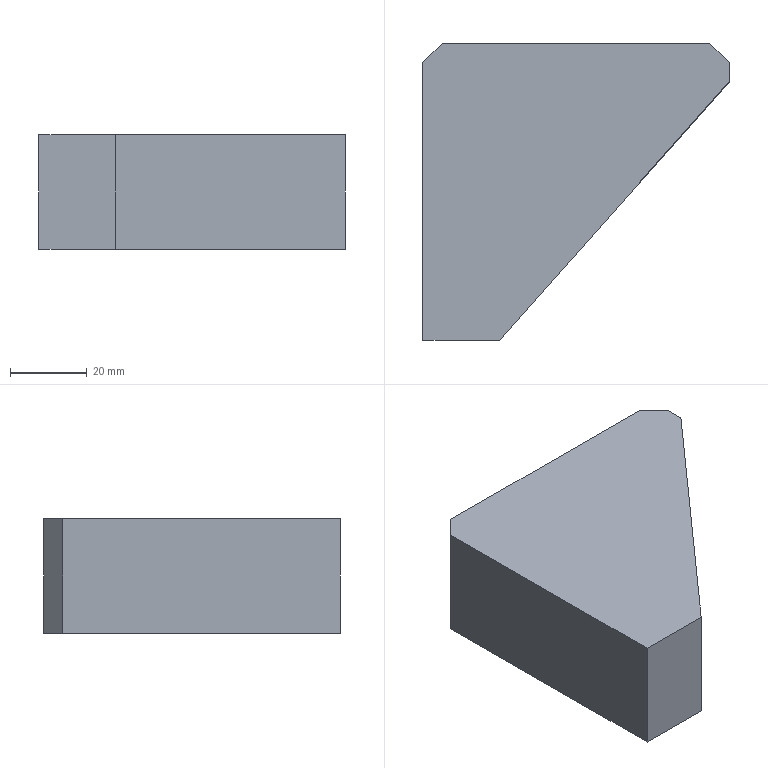Part | SolidWorks | features Extrusion 1 | 1 solid | 9 faces | box 80 x 77.5 x 30 mm | volume 124500 mm3 | plane 9
STEP:
#1=CARTESIAN_POINT('',(0.,0.,0.));
#2=VERTEX_POINT('',#1);
#3=CARTESIAN_POINT('',(20.,0.,0.));
#4=VERTEX_POINT('',#3);
#5=CARTESIAN_POINT('',(20.,0.,0.));
#6=DIRECTION('',(1.,0.,0.));
#7=VECTOR('',#6,1000.);
#8=LINE('',#5,#7);
#9=EDGE_CURVE('',#2,#4,#8,.T.);
#10=ORIENTED_EDGE('',*,*,#9,.T.);
#11=CARTESIAN_POINT('',(20.,0.,30.));
#12=VERTEX_POINT('',#11);
#13=CARTESIAN_POINT('',(20.,0.,30.));
#14=DIRECTION('',(0.,0.,-1.));
#15=VECTOR('',#14,1000.);
#16=LINE('',#13,#15);
#17=EDGE_CURVE('',#12,#4,#16,.T.);
#18=ORIENTED_EDGE('',*,*,#17,.F.);
#19=CARTESIAN_POINT('',(0.,0.,30.));
#20=VERTEX_POINT('',#19);
#21=CARTESIAN_POINT('',(20.,0.,30.));
#22=DIRECTION('',(1.,0.,0.));
#23=VECTOR('',#22,1000.);
#24=LINE('',#21,#23);
#25=EDGE_CURVE('',#20,#12,#24,.T.);
#26=ORIENTED_EDGE('',*,*,#25,.F.);
#27=CARTESIAN_POINT('',(0.,0.,30.));
#28=DIRECTION('',(0.,0.,-1.));
#29=VECTOR('',#28,1000.);
#30=LINE('',#27,#29);
#31=EDGE_CURVE('',#20,#2,#30,.T.);
#32=ORIENTED_EDGE('',*,*,#31,.T.);
#33=EDGE_LOOP('',(#10,#18,#26,#32));
#34=FACE_OUTER_BOUND('',#33,.T.);
#35=CARTESIAN_POINT('',(20.,0.,30.));
#36=DIRECTION('',(0.,1.,0.));
#37=DIRECTION('',(-1.,0.,0.));
#38=AXIS2_PLACEMENT_3D('',#35,#36,#37);
#39=PLANE('',#38);
#40=ADVANCED_FACE('',(#34),#39,.F.);
#41=CARTESIAN_POINT('',(80.,67.5,0.));
#42=VERTEX_POINT('',#41);
#43=CARTESIAN_POINT('',(80.,67.5,0.));
#44=DIRECTION('',(0.6644,0.7474,0.));
#45=VECTOR('',#44,1000.);
#46=LINE('',#43,#45);
#47=EDGE_CURVE('',#4,#42,#46,.T.);
#48=ORIENTED_EDGE('',*,*,#47,.T.);
#49=CARTESIAN_POINT('',(80.,67.5,30.));
#50=VERTEX_POINT('',#49);
#51=CARTESIAN_POINT('',(80.,67.5,30.));
#52=DIRECTION('',(0.,0.,-1.));
#53=VECTOR('',#52,1000.);
#54=LINE('',#51,#53);
#55=EDGE_CURVE('',#50,#42,#54,.T.);
#56=ORIENTED_EDGE('',*,*,#55,.F.);
#57=CARTESIAN_POINT('',(80.,67.5,30.));
#58=DIRECTION('',(0.6644,0.7474,0.));
#59=VECTOR('',#58,1000.);
#60=LINE('',#57,#59);
#61=EDGE_CURVE('',#12,#50,#60,.T.);
#62=ORIENTED_EDGE('',*,*,#61,.F.);
#63=ORIENTED_EDGE('',*,*,#17,.T.);
#64=EDGE_LOOP('',(#48,#56,#62,#63));
#65=FACE_OUTER_BOUND('',#64,.T.);
#66=CARTESIAN_POINT('',(80.,67.5,30.));
#67=DIRECTION('',(-0.7474,0.6644,0.));
#68=DIRECTION('',(-0.6644,-0.7474,0.));
#69=AXIS2_PLACEMENT_3D('',#66,#67,#68);
#70=PLANE('',#69);
#71=ADVANCED_FACE('',(#65),#70,.F.);
#72=CARTESIAN_POINT('',(80.,72.5,0.));
#73=VERTEX_POINT('',#72);
#74=CARTESIAN_POINT('',(80.,72.5,0.));
#75=DIRECTION('',(0.,1.,0.));
#76=VECTOR('',#75,1000.);
#77=LINE('',#74,#76);
#78=EDGE_CURVE('',#42,#73,#77,.T.);
#79=ORIENTED_EDGE('',*,*,#78,.T.);
#80=CARTESIAN_POINT('',(80.,72.5,30.));
#81=VERTEX_POINT('',#80);
#82=CARTESIAN_POINT('',(80.,72.5,30.));
#83=DIRECTION('',(0.,0.,-1.));
#84=VECTOR('',#83,1000.);
#85=LINE('',#82,#84);
#86=EDGE_CURVE('',#81,#73,#85,.T.);
#87=ORIENTED_EDGE('',*,*,#86,.F.);
#88=CARTESIAN_POINT('',(80.,72.5,30.));
#89=DIRECTION('',(0.,1.,0.));
#90=VECTOR('',#89,1000.);
#91=LINE('',#88,#90);
#92=EDGE_CURVE('',#50,#81,#91,.T.);
#93=ORIENTED_EDGE('',*,*,#92,.F.);
#94=ORIENTED_EDGE('',*,*,#55,.T.);
#95=EDGE_LOOP('',(#79,#87,#93,#94));
#96=FACE_OUTER_BOUND('',#95,.T.);
#97=CARTESIAN_POINT('',(80.,72.5,30.));
#98=DIRECTION('',(-1.,0.,0.));
#99=DIRECTION('',(0.,0.,1.));
#100=AXIS2_PLACEMENT_3D('',#97,#98,#99);
#101=PLANE('',#100);
#102=ADVANCED_FACE('',(#96),#101,.F.);
#103=CARTESIAN_POINT('',(75.,77.5,0.));
#104=VERTEX_POINT('',#103);
#105=CARTESIAN_POINT('',(75.,77.5,0.));
#106=DIRECTION('',(-0.7071,0.7071,0.));
#107=VECTOR('',#106,1000.);
#108=LINE('',#105,#107);
#109=EDGE_CURVE('',#73,#104,#108,.T.);
#110=ORIENTED_EDGE('',*,*,#109,.T.);
#111=CARTESIAN_POINT('',(75.,77.5,30.));
#112=VERTEX_POINT('',#111);
#113=CARTESIAN_POINT('',(75.,77.5,30.));
#114=DIRECTION('',(0.,0.,-1.));
#115=VECTOR('',#114,1000.);
#116=LINE('',#113,#115);
#117=EDGE_CURVE('',#112,#104,#116,.T.);
#118=ORIENTED_EDGE('',*,*,#117,.F.);
#119=CARTESIAN_POINT('',(75.,77.5,30.));
#120=DIRECTION('',(-0.7071,0.7071,0.));
#121=VECTOR('',#120,1000.);
#122=LINE('',#119,#121);
#123=EDGE_CURVE('',#81,#112,#122,.T.);
#124=ORIENTED_EDGE('',*,*,#123,.F.);
#125=ORIENTED_EDGE('',*,*,#86,.T.);
#126=EDGE_LOOP('',(#110,#118,#124,#125));
#127=FACE_OUTER_BOUND('',#126,.T.);
#128=CARTESIAN_POINT('',(75.,77.5,30.));
#129=DIRECTION('',(-0.7071,-0.7071,0.));
#130=DIRECTION('',(0.7071,-0.7071,0.));
#131=AXIS2_PLACEMENT_3D('',#128,#129,#130);
#132=PLANE('',#131);
#133=ADVANCED_FACE('',(#127),#132,.F.);
#134=CARTESIAN_POINT('',(5.,77.5,0.));
#135=VERTEX_POINT('',#134);
#136=CARTESIAN_POINT('',(5.,77.5,0.));
#137=DIRECTION('',(-1.,0.,0.));
#138=VECTOR('',#137,1000.);
#139=LINE('',#136,#138);
#140=EDGE_CURVE('',#104,#135,#139,.T.);
#141=ORIENTED_EDGE('',*,*,#140,.T.);
#142=CARTESIAN_POINT('',(5.,77.5,30.));
#143=VERTEX_POINT('',#142);
#144=CARTESIAN_POINT('',(5.,77.5,30.));
#145=DIRECTION('',(0.,0.,-1.));
#146=VECTOR('',#145,1000.);
#147=LINE('',#144,#146);
#148=EDGE_CURVE('',#143,#135,#147,.T.);
#149=ORIENTED_EDGE('',*,*,#148,.F.);
#150=CARTESIAN_POINT('',(5.,77.5,30.));
#151=DIRECTION('',(-1.,0.,0.));
#152=VECTOR('',#151,1000.);
#153=LINE('',#150,#152);
#154=EDGE_CURVE('',#112,#143,#153,.T.);
#155=ORIENTED_EDGE('',*,*,#154,.F.);
#156=ORIENTED_EDGE('',*,*,#117,.T.);
#157=EDGE_LOOP('',(#141,#149,#155,#156));
#158=FACE_OUTER_BOUND('',#157,.T.);
#159=CARTESIAN_POINT('',(5.,77.5,30.));
#160=DIRECTION('',(0.,-1.,0.));
#161=DIRECTION('',(0.,0.,-1.));
#162=AXIS2_PLACEMENT_3D('',#159,#160,#161);
#163=PLANE('',#162);
#164=ADVANCED_FACE('',(#158),#163,.F.);
#165=CARTESIAN_POINT('',(0.,72.5,0.));
#166=VERTEX_POINT('',#165);
#167=CARTESIAN_POINT('',(0.,72.5,0.));
#168=DIRECTION('',(-0.7071,-0.7071,0.));
#169=VECTOR('',#168,1000.);
#170=LINE('',#167,#169);
#171=EDGE_CURVE('',#135,#166,#170,.T.);
#172=ORIENTED_EDGE('',*,*,#171,.T.);
#173=CARTESIAN_POINT('',(0.,72.5,30.));
#174=VERTEX_POINT('',#173);
#175=CARTESIAN_POINT('',(0.,72.5,30.));
#176=DIRECTION('',(0.,0.,-1.));
#177=VECTOR('',#176,1000.);
#178=LINE('',#175,#177);
#179=EDGE_CURVE('',#174,#166,#178,.T.);
#180=ORIENTED_EDGE('',*,*,#179,.F.);
#181=CARTESIAN_POINT('',(0.,72.5,30.));
#182=DIRECTION('',(-0.7071,-0.7071,0.));
#183=VECTOR('',#182,1000.);
#184=LINE('',#181,#183);
#185=EDGE_CURVE('',#143,#174,#184,.T.);
#186=ORIENTED_EDGE('',*,*,#185,.F.);
#187=ORIENTED_EDGE('',*,*,#148,.T.);
#188=EDGE_LOOP('',(#172,#180,#186,#187));
#189=FACE_OUTER_BOUND('',#188,.T.);
#190=CARTESIAN_POINT('',(0.,72.5,30.));
#191=DIRECTION('',(0.7071,-0.7071,0.));
#192=DIRECTION('',(0.7071,0.7071,0.));
#193=AXIS2_PLACEMENT_3D('',#190,#191,#192);
#194=PLANE('',#193);
#195=ADVANCED_FACE('',(#189),#194,.F.);
#196=CARTESIAN_POINT('',(0.,0.,0.));
#197=DIRECTION('',(0.,-1.,0.));
#198=VECTOR('',#197,1000.);
#199=LINE('',#196,#198);
#200=EDGE_CURVE('',#166,#2,#199,.T.);
#201=ORIENTED_EDGE('',*,*,#200,.T.);
#202=ORIENTED_EDGE('',*,*,#31,.F.);
#203=CARTESIAN_POINT('',(0.,0.,30.));
#204=DIRECTION('',(0.,-1.,0.));
#205=VECTOR('',#204,1000.);
#206=LINE('',#203,#205);
#207=EDGE_CURVE('',#174,#20,#206,.T.);
#208=ORIENTED_EDGE('',*,*,#207,.F.);
#209=ORIENTED_EDGE('',*,*,#179,.T.);
#210=EDGE_LOOP('',(#201,#202,#208,#209));
#211=FACE_OUTER_BOUND('',#210,.T.);
#212=CARTESIAN_POINT('',(0.,0.,30.));
#213=DIRECTION('',(1.,0.,0.));
#214=DIRECTION('',(0.,0.,-1.));
#215=AXIS2_PLACEMENT_3D('',#212,#213,#214);
#216=PLANE('',#215);
#217=ADVANCED_FACE('',(#211),#216,.F.);
#218=ORIENTED_EDGE('',*,*,#25,.T.);
#219=ORIENTED_EDGE('',*,*,#61,.T.);
#220=ORIENTED_EDGE('',*,*,#92,.T.);
#221=ORIENTED_EDGE('',*,*,#123,.T.);
#222=ORIENTED_EDGE('',*,*,#154,.T.);
#223=ORIENTED_EDGE('',*,*,#185,.T.);
#224=ORIENTED_EDGE('',*,*,#207,.T.);
#225=EDGE_LOOP('',(#218,#219,#220,#221,#222,#223,#224));
#226=FACE_OUTER_BOUND('',#225,.T.);
#227=CARTESIAN_POINT('',(0.,0.,30.));
#228=DIRECTION('',(0.,0.,-1.));
#229=DIRECTION('',(-1.,0.,0.));
#230=AXIS2_PLACEMENT_3D('',#227,#228,#229);
#231=PLANE('',#230);
#232=ADVANCED_FACE('',(#226),#231,.F.);
#233=ORIENTED_EDGE('',*,*,#9,.F.);
#234=ORIENTED_EDGE('',*,*,#200,.F.);
#235=ORIENTED_EDGE('',*,*,#171,.F.);
#236=ORIENTED_EDGE('',*,*,#140,.F.);
#237=ORIENTED_EDGE('',*,*,#109,.F.);
#238=ORIENTED_EDGE('',*,*,#78,.F.);
#239=ORIENTED_EDGE('',*,*,#47,.F.);
#240=EDGE_LOOP('',(#233,#234,#235,#236,#237,#238,#239));
#241=FACE_OUTER_BOUND('',#240,.T.);
#242=CARTESIAN_POINT('',(0.,0.,0.));
#243=DIRECTION('',(0.,0.,-1.));
#244=DIRECTION('',(-1.,0.,0.));
#245=AXIS2_PLACEMENT_3D('',#242,#243,#244);
#246=PLANE('',#245);
#247=ADVANCED_FACE('',(#241),#246,.T.);
#248=CLOSED_SHELL('',(#40,#71,#102,#133,#164,#195,#217,#232,#247));
#249=MANIFOLD_SOLID_BREP('',#248);
#250=CARTESIAN_POINT('',(0.,0.,0.));
#251=DIRECTION('',(0.,0.,1.));
#252=DIRECTION('',(1.,0.,0.));
#253=AXIS2_PLACEMENT_3D('',#250,#251,#252);
#254=(LENGTH_UNIT()NAMED_UNIT(*)SI_UNIT(.MILLI.,.METRE.));
#255=UNCERTAINTY_MEASURE_WITH_UNIT(LENGTH_MEASURE(0.00001),#254,'','');
#256=(NAMED_UNIT(*)PLANE_ANGLE_UNIT()SI_UNIT($,.RADIAN.));
#257=(NAMED_UNIT(*)SI_UNIT($,.STERADIAN.)SOLID_ANGLE_UNIT());
#258=(GEOMETRIC_REPRESENTATION_CONTEXT(3)GLOBAL_UNCERTAINTY_ASSIGNED_CONTEXT((#255))GLOBAL_UNIT_ASSIGNED_CONTEXT((#254,#256,#257))REPRESENTATION_CONTEXT('',''));
#259=ADVANCED_BREP_SHAPE_REPRESENTATION('',(#249,#253),#258);